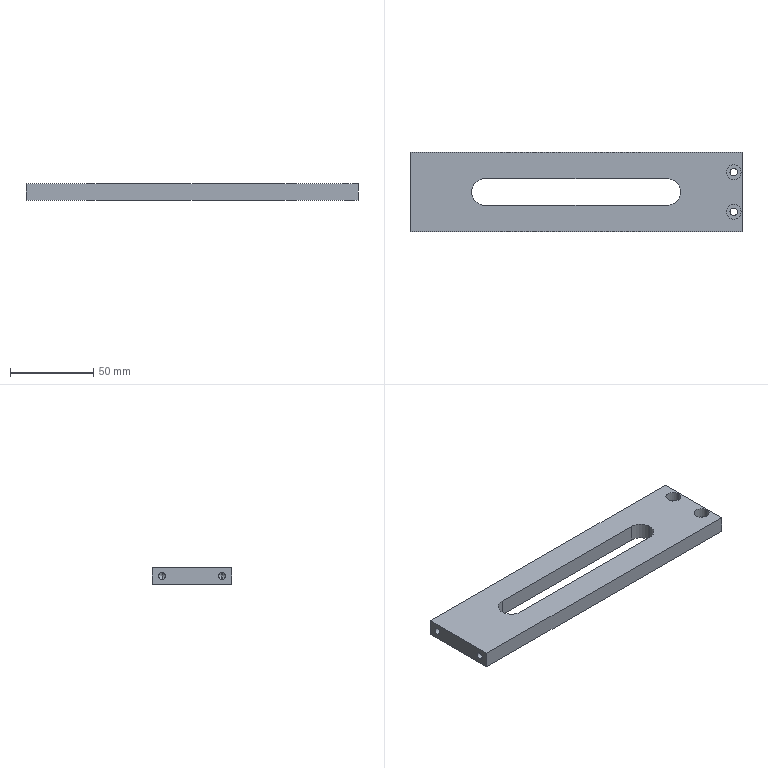Part | STEP file | B1-006 | 1 solid | 29 faces | box 200 x 48 x 10 mm | volume 75143 mm3 | cylinder 15 | plane 10 | cone 4 | commonest cylinder face diameters 4.2 x4 4.5 x4 9 x4 16 x3